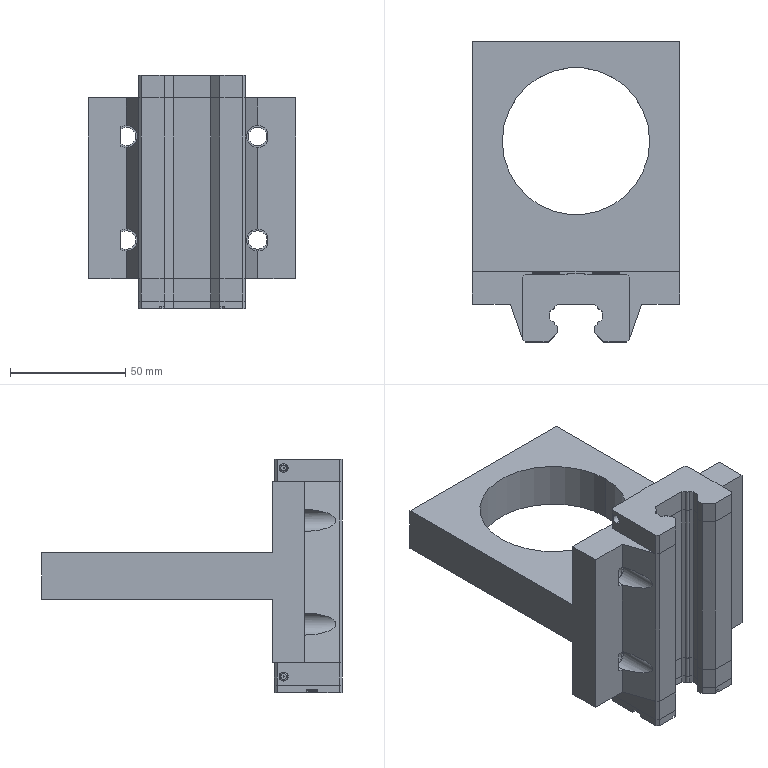Part | STEP file | 4 solids | 301 faces | box 90 x 130.4 x 101.35 mm | volume 273485 mm3 | plane 211 | cylinder 76 | spline 14 | commonest cylinder face diameters 2.258 x24 9.6 x13 3.9 x12 8 x10 0.526 x8 3.724 x4